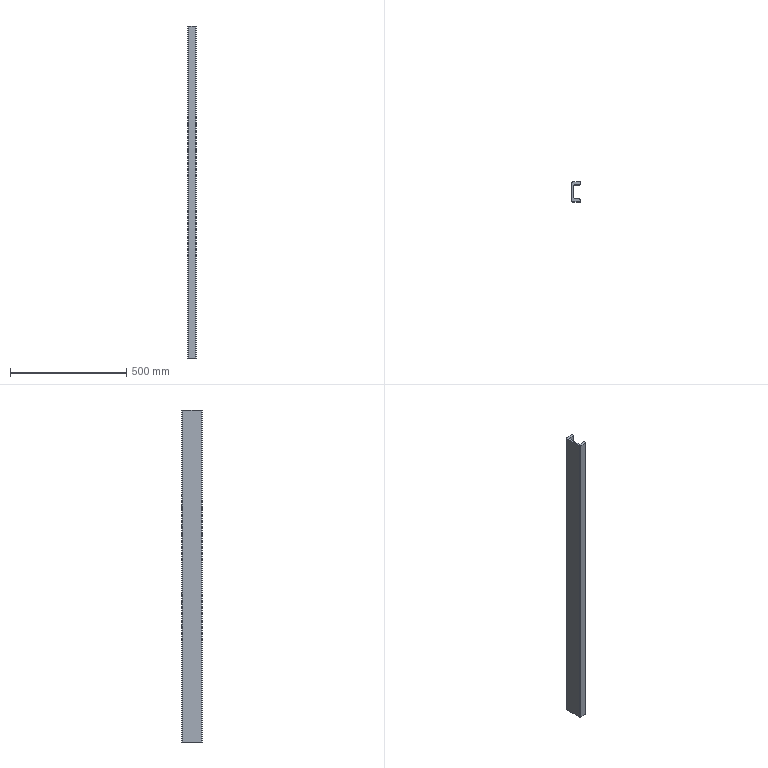Part | SolidWorks | features Extrusion 1, HoleWzd 1 | 1 solid | 42 faces | box 36 x 86.5 x 1430 mm | volume 1904339 mm3 | cylinder 22 | plane 12 | cone 8 | commonest cylinder face diameters 5 x18 6 x2 8 x2